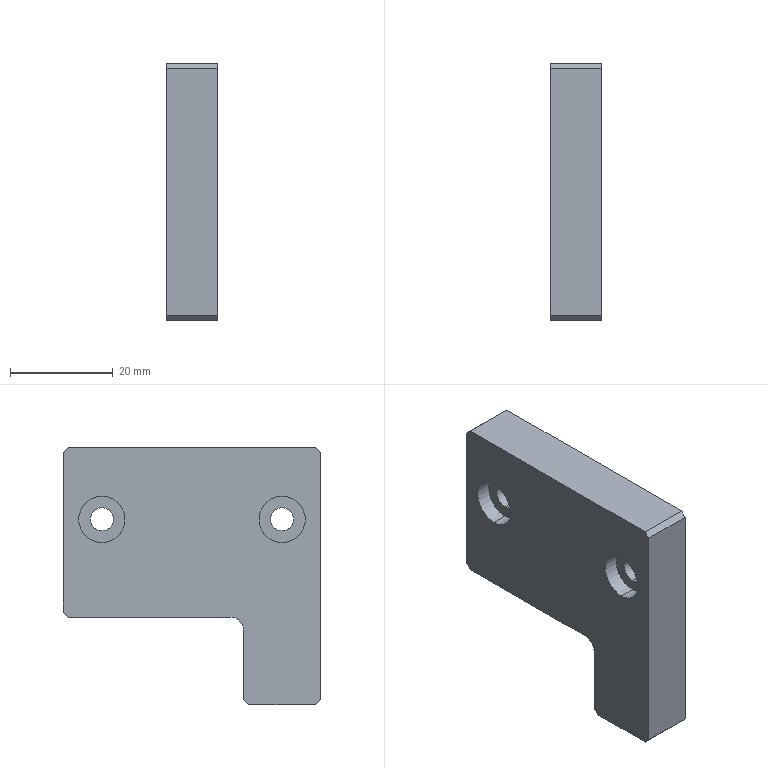Part | STEP file | Fixing plate 3 | 1 solid | 34 faces | box 10 x 50 x 50 mm | volume 18064 mm3 | plane 17 | cylinder 15 | cone 2 | commonest cylinder face diameters 9 x8 4.5 x4 3.3 x2 5 x1